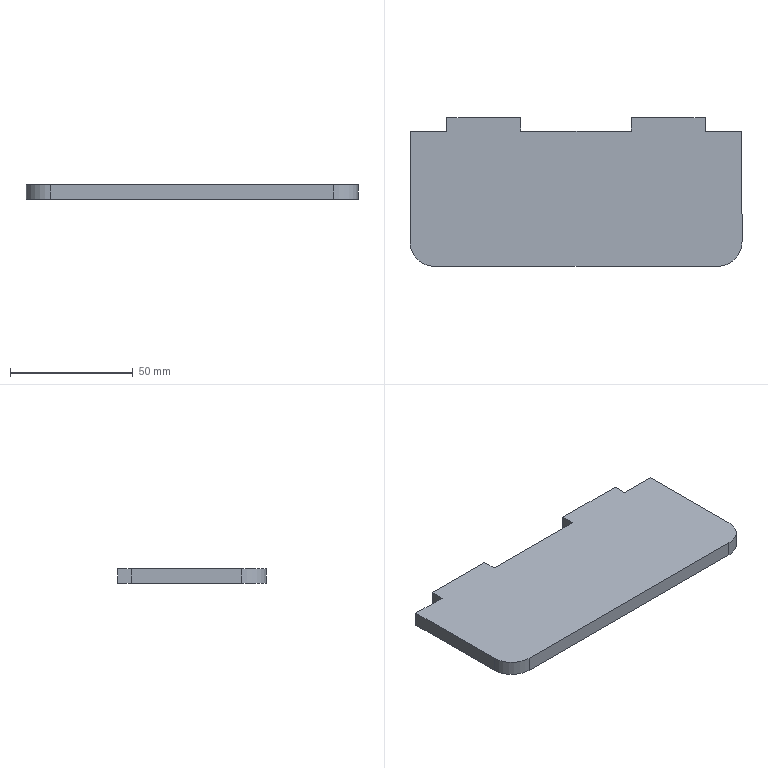Part | SolidWorks | features FlatPattern 1, SMBaseFlange 1, SheetMetal 1 | 1 solid | 16 faces | box 135 x 60.5 x 6 mm | volume 46272 mm3 | plane 14 | cylinder 2 | commonest cylinder face diameters 20 x2
STEP:
#1=CARTESIAN_POINT('',(128.47,-600.5,0.));
#2=VERTEX_POINT('',#1);
#3=CARTESIAN_POINT('',(128.47,-555.5,0.));
#4=VERTEX_POINT('',#3);
#5=CARTESIAN_POINT('',(128.47,-555.5,0.));
#6=DIRECTION('',(0.,1.,0.));
#7=VECTOR('',#6,1000.);
#8=LINE('',#5,#7);
#9=EDGE_CURVE('',#2,#4,#8,.T.);
#10=ORIENTED_EDGE('',*,*,#9,.F.);
#11=CARTESIAN_POINT('',(128.47,-600.5,-6.));
#12=VERTEX_POINT('',#11);
#13=CARTESIAN_POINT('',(128.47,-600.5,-6.));
#14=DIRECTION('',(0.,0.,1.));
#15=VECTOR('',#14,1000.);
#16=LINE('',#13,#15);
#17=EDGE_CURVE('',#12,#2,#16,.T.);
#18=ORIENTED_EDGE('',*,*,#17,.F.);
#19=CARTESIAN_POINT('',(128.47,-555.5,-6.));
#20=VERTEX_POINT('',#19);
#21=CARTESIAN_POINT('',(128.47,-555.5,-6.));
#22=DIRECTION('',(0.,1.,0.));
#23=VECTOR('',#22,1000.);
#24=LINE('',#21,#23);
#25=EDGE_CURVE('',#12,#20,#24,.T.);
#26=ORIENTED_EDGE('',*,*,#25,.T.);
#27=CARTESIAN_POINT('',(128.47,-555.5,-6.));
#28=DIRECTION('',(0.,0.,1.));
#29=VECTOR('',#28,1000.);
#30=LINE('',#27,#29);
#31=EDGE_CURVE('',#20,#4,#30,.T.);
#32=ORIENTED_EDGE('',*,*,#31,.T.);
#33=EDGE_LOOP('',(#10,#18,#26,#32));
#34=FACE_OUTER_BOUND('',#33,.T.);
#35=CARTESIAN_POINT('',(128.47,-555.5,-6.));
#36=DIRECTION('',(1.,0.,0.));
#37=DIRECTION('',(0.,1.,0.));
#38=AXIS2_PLACEMENT_3D('',#35,#36,#37);
#39=PLANE('',#38);
#40=ADVANCED_FACE('',(#34),#39,.T.);
#41=CARTESIAN_POINT('',(118.47,-610.5,0.));
#42=VERTEX_POINT('',#41);
#43=CARTESIAN_POINT('',(118.47,-600.5,0.));
#44=DIRECTION('',(0.,0.,1.));
#45=DIRECTION('',(-1.,0.,0.));
#46=AXIS2_PLACEMENT_3D('',#43,#44,#45);
#47=CIRCLE('',#46,10.);
#48=EDGE_CURVE('',#42,#2,#47,.T.);
#49=ORIENTED_EDGE('',*,*,#48,.F.);
#50=CARTESIAN_POINT('',(118.47,-610.5,-6.));
#51=VERTEX_POINT('',#50);
#52=CARTESIAN_POINT('',(118.47,-610.5,-6.));
#53=DIRECTION('',(0.,0.,1.));
#54=VECTOR('',#53,1000.);
#55=LINE('',#52,#54);
#56=EDGE_CURVE('',#51,#42,#55,.T.);
#57=ORIENTED_EDGE('',*,*,#56,.F.);
#58=CARTESIAN_POINT('',(118.47,-600.5,-6.));
#59=DIRECTION('',(0.,0.,1.));
#60=DIRECTION('',(-1.,0.,0.));
#61=AXIS2_PLACEMENT_3D('',#58,#59,#60);
#62=CIRCLE('',#61,10.);
#63=EDGE_CURVE('',#51,#12,#62,.T.);
#64=ORIENTED_EDGE('',*,*,#63,.T.);
#65=ORIENTED_EDGE('',*,*,#17,.T.);
#66=EDGE_LOOP('',(#49,#57,#64,#65));
#67=FACE_OUTER_BOUND('',#66,.T.);
#68=CARTESIAN_POINT('',(118.47,-600.5,-6.));
#69=DIRECTION('',(0.,0.,1.));
#70=DIRECTION('',(1.,0.,0.));
#71=AXIS2_PLACEMENT_3D('',#68,#69,#70);
#72=CYLINDRICAL_SURFACE('',#71,10.);
#73=ADVANCED_FACE('',(#67),#72,.T.);
#74=CARTESIAN_POINT('',(3.47,-610.5,0.));
#75=VERTEX_POINT('',#74);
#76=CARTESIAN_POINT('',(118.47,-610.5,0.));
#77=DIRECTION('',(1.,0.,0.));
#78=VECTOR('',#77,1000.);
#79=LINE('',#76,#78);
#80=EDGE_CURVE('',#75,#42,#79,.T.);
#81=ORIENTED_EDGE('',*,*,#80,.F.);
#82=CARTESIAN_POINT('',(3.47,-610.5,-6.));
#83=VERTEX_POINT('',#82);
#84=CARTESIAN_POINT('',(3.47,-610.5,-6.));
#85=DIRECTION('',(0.,0.,1.));
#86=VECTOR('',#85,1000.);
#87=LINE('',#84,#86);
#88=EDGE_CURVE('',#83,#75,#87,.T.);
#89=ORIENTED_EDGE('',*,*,#88,.F.);
#90=CARTESIAN_POINT('',(118.47,-610.5,-6.));
#91=DIRECTION('',(1.,0.,0.));
#92=VECTOR('',#91,1000.);
#93=LINE('',#90,#92);
#94=EDGE_CURVE('',#83,#51,#93,.T.);
#95=ORIENTED_EDGE('',*,*,#94,.T.);
#96=ORIENTED_EDGE('',*,*,#56,.T.);
#97=EDGE_LOOP('',(#81,#89,#95,#96));
#98=FACE_OUTER_BOUND('',#97,.T.);
#99=CARTESIAN_POINT('',(118.47,-610.5,-6.));
#100=DIRECTION('',(0.,-1.,0.));
#101=DIRECTION('',(1.,0.,0.));
#102=AXIS2_PLACEMENT_3D('',#99,#100,#101);
#103=PLANE('',#102);
#104=ADVANCED_FACE('',(#98),#103,.T.);
#105=CARTESIAN_POINT('',(-6.53,-600.5,0.));
#106=VERTEX_POINT('',#105);
#107=CARTESIAN_POINT('',(3.47,-600.5,0.));
#108=DIRECTION('',(0.,0.,1.));
#109=DIRECTION('',(-1.,0.,0.));
#110=AXIS2_PLACEMENT_3D('',#107,#108,#109);
#111=CIRCLE('',#110,10.);
#112=EDGE_CURVE('',#106,#75,#111,.T.);
#113=ORIENTED_EDGE('',*,*,#112,.F.);
#114=CARTESIAN_POINT('',(-6.53,-600.5,-6.));
#115=VERTEX_POINT('',#114);
#116=CARTESIAN_POINT('',(-6.53,-600.5,-6.));
#117=DIRECTION('',(0.,0.,1.));
#118=VECTOR('',#117,1000.);
#119=LINE('',#116,#118);
#120=EDGE_CURVE('',#115,#106,#119,.T.);
#121=ORIENTED_EDGE('',*,*,#120,.F.);
#122=CARTESIAN_POINT('',(3.47,-600.5,-6.));
#123=DIRECTION('',(0.,0.,1.));
#124=DIRECTION('',(-1.,0.,0.));
#125=AXIS2_PLACEMENT_3D('',#122,#123,#124);
#126=CIRCLE('',#125,10.);
#127=EDGE_CURVE('',#115,#83,#126,.T.);
#128=ORIENTED_EDGE('',*,*,#127,.T.);
#129=ORIENTED_EDGE('',*,*,#88,.T.);
#130=EDGE_LOOP('',(#113,#121,#128,#129));
#131=FACE_OUTER_BOUND('',#130,.T.);
#132=CARTESIAN_POINT('',(3.47,-600.5,-6.));
#133=DIRECTION('',(0.,0.,1.));
#134=DIRECTION('',(1.,0.,0.));
#135=AXIS2_PLACEMENT_3D('',#132,#133,#134);
#136=CYLINDRICAL_SURFACE('',#135,10.);
#137=ADVANCED_FACE('',(#131),#136,.T.);
#138=CARTESIAN_POINT('',(-6.53,-555.5,0.));
#139=VERTEX_POINT('',#138);
#140=CARTESIAN_POINT('',(-6.53,-555.5,0.));
#141=DIRECTION('',(0.,-1.,0.));
#142=VECTOR('',#141,1000.);
#143=LINE('',#140,#142);
#144=EDGE_CURVE('',#139,#106,#143,.T.);
#145=ORIENTED_EDGE('',*,*,#144,.F.);
#146=CARTESIAN_POINT('',(-6.53,-555.5,-6.));
#147=VERTEX_POINT('',#146);
#148=CARTESIAN_POINT('',(-6.53,-555.5,-6.));
#149=DIRECTION('',(0.,0.,1.));
#150=VECTOR('',#149,1000.);
#151=LINE('',#148,#150);
#152=EDGE_CURVE('',#147,#139,#151,.T.);
#153=ORIENTED_EDGE('',*,*,#152,.F.);
#154=CARTESIAN_POINT('',(-6.53,-555.5,-6.));
#155=DIRECTION('',(0.,-1.,0.));
#156=VECTOR('',#155,1000.);
#157=LINE('',#154,#156);
#158=EDGE_CURVE('',#147,#115,#157,.T.);
#159=ORIENTED_EDGE('',*,*,#158,.T.);
#160=ORIENTED_EDGE('',*,*,#120,.T.);
#161=EDGE_LOOP('',(#145,#153,#159,#160));
#162=FACE_OUTER_BOUND('',#161,.T.);
#163=CARTESIAN_POINT('',(-6.53,-555.5,-6.));
#164=DIRECTION('',(-1.,0.,0.));
#165=DIRECTION('',(0.,-1.,0.));
#166=AXIS2_PLACEMENT_3D('',#163,#164,#165);
#167=PLANE('',#166);
#168=ADVANCED_FACE('',(#162),#167,.T.);
#169=CARTESIAN_POINT('',(8.47,-555.5,0.));
#170=VERTEX_POINT('',#169);
#171=CARTESIAN_POINT('',(8.47,-555.5,0.));
#172=DIRECTION('',(-1.,0.,0.));
#173=VECTOR('',#172,1000.);
#174=LINE('',#171,#173);
#175=EDGE_CURVE('',#170,#139,#174,.T.);
#176=ORIENTED_EDGE('',*,*,#175,.F.);
#177=CARTESIAN_POINT('',(8.47,-555.5,-6.));
#178=VERTEX_POINT('',#177);
#179=CARTESIAN_POINT('',(8.47,-555.5,-6.));
#180=DIRECTION('',(0.,0.,1.));
#181=VECTOR('',#180,1000.);
#182=LINE('',#179,#181);
#183=EDGE_CURVE('',#178,#170,#182,.T.);
#184=ORIENTED_EDGE('',*,*,#183,.F.);
#185=CARTESIAN_POINT('',(8.47,-555.5,-6.));
#186=DIRECTION('',(-1.,0.,0.));
#187=VECTOR('',#186,1000.);
#188=LINE('',#185,#187);
#189=EDGE_CURVE('',#178,#147,#188,.T.);
#190=ORIENTED_EDGE('',*,*,#189,.T.);
#191=ORIENTED_EDGE('',*,*,#152,.T.);
#192=EDGE_LOOP('',(#176,#184,#190,#191));
#193=FACE_OUTER_BOUND('',#192,.T.);
#194=CARTESIAN_POINT('',(8.47,-555.5,-6.));
#195=DIRECTION('',(0.,1.,0.));
#196=DIRECTION('',(0.,0.,1.));
#197=AXIS2_PLACEMENT_3D('',#194,#195,#196);
#198=PLANE('',#197);
#199=ADVANCED_FACE('',(#193),#198,.T.);
#200=CARTESIAN_POINT('',(8.47,-550.,0.));
#201=VERTEX_POINT('',#200);
#202=CARTESIAN_POINT('',(8.47,-550.,0.));
#203=DIRECTION('',(0.,-1.,0.));
#204=VECTOR('',#203,1000.);
#205=LINE('',#202,#204);
#206=EDGE_CURVE('',#201,#170,#205,.T.);
#207=ORIENTED_EDGE('',*,*,#206,.F.);
#208=CARTESIAN_POINT('',(8.47,-550.,-6.));
#209=VERTEX_POINT('',#208);
#210=CARTESIAN_POINT('',(8.47,-550.,-6.));
#211=DIRECTION('',(0.,0.,1.));
#212=VECTOR('',#211,1000.);
#213=LINE('',#210,#212);
#214=EDGE_CURVE('',#209,#201,#213,.T.);
#215=ORIENTED_EDGE('',*,*,#214,.F.);
#216=CARTESIAN_POINT('',(8.47,-550.,-6.));
#217=DIRECTION('',(0.,-1.,0.));
#218=VECTOR('',#217,1000.);
#219=LINE('',#216,#218);
#220=EDGE_CURVE('',#209,#178,#219,.T.);
#221=ORIENTED_EDGE('',*,*,#220,.T.);
#222=ORIENTED_EDGE('',*,*,#183,.T.);
#223=EDGE_LOOP('',(#207,#215,#221,#222));
#224=FACE_OUTER_BOUND('',#223,.T.);
#225=CARTESIAN_POINT('',(8.47,-550.,-6.));
#226=DIRECTION('',(-1.,0.,0.));
#227=DIRECTION('',(0.,0.,1.));
#228=AXIS2_PLACEMENT_3D('',#225,#226,#227);
#229=PLANE('',#228);
#230=ADVANCED_FACE('',(#224),#229,.T.);
#231=CARTESIAN_POINT('',(38.47,-550.,0.));
#232=VERTEX_POINT('',#231);
#233=CARTESIAN_POINT('',(38.47,-550.,0.));
#234=DIRECTION('',(-1.,0.,0.));
#235=VECTOR('',#234,1000.);
#236=LINE('',#233,#235);
#237=EDGE_CURVE('',#232,#201,#236,.T.);
#238=ORIENTED_EDGE('',*,*,#237,.F.);
#239=CARTESIAN_POINT('',(38.47,-550.,-6.));
#240=VERTEX_POINT('',#239);
#241=CARTESIAN_POINT('',(38.47,-550.,-6.));
#242=DIRECTION('',(0.,0.,1.));
#243=VECTOR('',#242,1000.);
#244=LINE('',#241,#243);
#245=EDGE_CURVE('',#240,#232,#244,.T.);
#246=ORIENTED_EDGE('',*,*,#245,.F.);
#247=CARTESIAN_POINT('',(38.47,-550.,-6.));
#248=DIRECTION('',(-1.,0.,0.));
#249=VECTOR('',#248,1000.);
#250=LINE('',#247,#249);
#251=EDGE_CURVE('',#240,#209,#250,.T.);
#252=ORIENTED_EDGE('',*,*,#251,.T.);
#253=ORIENTED_EDGE('',*,*,#214,.T.);
#254=EDGE_LOOP('',(#238,#246,#252,#253));
#255=FACE_OUTER_BOUND('',#254,.T.);
#256=CARTESIAN_POINT('',(38.47,-550.,-6.));
#257=DIRECTION('',(0.,1.,0.));
#258=DIRECTION('',(0.,0.,1.));
#259=AXIS2_PLACEMENT_3D('',#256,#257,#258);
#260=PLANE('',#259);
#261=ADVANCED_FACE('',(#255),#260,.T.);
#262=CARTESIAN_POINT('',(38.47,-555.5,0.));
#263=VERTEX_POINT('',#262);
#264=CARTESIAN_POINT('',(38.47,-555.5,0.));
#265=DIRECTION('',(0.,1.,0.));
#266=VECTOR('',#265,1000.);
#267=LINE('',#264,#266);
#268=EDGE_CURVE('',#263,#232,#267,.T.);
#269=ORIENTED_EDGE('',*,*,#268,.F.);
#270=CARTESIAN_POINT('',(38.47,-555.5,-6.));
#271=VERTEX_POINT('',#270);
#272=CARTESIAN_POINT('',(38.47,-555.5,-6.));
#273=DIRECTION('',(0.,0.,1.));
#274=VECTOR('',#273,1000.);
#275=LINE('',#272,#274);
#276=EDGE_CURVE('',#271,#263,#275,.T.);
#277=ORIENTED_EDGE('',*,*,#276,.F.);
#278=CARTESIAN_POINT('',(38.47,-555.5,-6.));
#279=DIRECTION('',(0.,1.,0.));
#280=VECTOR('',#279,1000.);
#281=LINE('',#278,#280);
#282=EDGE_CURVE('',#271,#240,#281,.T.);
#283=ORIENTED_EDGE('',*,*,#282,.T.);
#284=ORIENTED_EDGE('',*,*,#245,.T.);
#285=EDGE_LOOP('',(#269,#277,#283,#284));
#286=FACE_OUTER_BOUND('',#285,.T.);
#287=CARTESIAN_POINT('',(38.47,-555.5,-6.));
#288=DIRECTION('',(1.,0.,0.));
#289=DIRECTION('',(0.,0.,-1.));
#290=AXIS2_PLACEMENT_3D('',#287,#288,#289);
#291=PLANE('',#290);
#292=ADVANCED_FACE('',(#286),#291,.T.);
#293=CARTESIAN_POINT('',(83.47,-555.5,0.));
#294=VERTEX_POINT('',#293);
#295=CARTESIAN_POINT('',(83.47,-555.5,0.));
#296=DIRECTION('',(-1.,0.,0.));
#297=VECTOR('',#296,1000.);
#298=LINE('',#295,#297);
#299=EDGE_CURVE('',#294,#263,#298,.T.);
#300=ORIENTED_EDGE('',*,*,#299,.F.);
#301=CARTESIAN_POINT('',(83.47,-555.5,-6.));
#302=VERTEX_POINT('',#301);
#303=CARTESIAN_POINT('',(83.47,-555.5,-6.));
#304=DIRECTION('',(0.,0.,1.));
#305=VECTOR('',#304,1000.);
#306=LINE('',#303,#305);
#307=EDGE_CURVE('',#302,#294,#306,.T.);
#308=ORIENTED_EDGE('',*,*,#307,.F.);
#309=CARTESIAN_POINT('',(83.47,-555.5,-6.));
#310=DIRECTION('',(-1.,0.,0.));
#311=VECTOR('',#310,1000.);
#312=LINE('',#309,#311);
#313=EDGE_CURVE('',#302,#271,#312,.T.);
#314=ORIENTED_EDGE('',*,*,#313,.T.);
#315=ORIENTED_EDGE('',*,*,#276,.T.);
#316=EDGE_LOOP('',(#300,#308,#314,#315));
#317=FACE_OUTER_BOUND('',#316,.T.);
#318=CARTESIAN_POINT('',(83.47,-555.5,-6.));
#319=DIRECTION('',(0.,1.,0.));
#320=DIRECTION('',(0.,0.,1.));
#321=AXIS2_PLACEMENT_3D('',#318,#319,#320);
#322=PLANE('',#321);
#323=ADVANCED_FACE('',(#317),#322,.T.);
#324=CARTESIAN_POINT('',(83.47,-550.,0.));
#325=VERTEX_POINT('',#324);
#326=CARTESIAN_POINT('',(83.47,-550.,0.));
#327=DIRECTION('',(0.,-1.,0.));
#328=VECTOR('',#327,1000.);
#329=LINE('',#326,#328);
#330=EDGE_CURVE('',#325,#294,#329,.T.);
#331=ORIENTED_EDGE('',*,*,#330,.F.);
#332=CARTESIAN_POINT('',(83.47,-550.,-6.));
#333=VERTEX_POINT('',#332);
#334=CARTESIAN_POINT('',(83.47,-550.,-6.));
#335=DIRECTION('',(0.,0.,1.));
#336=VECTOR('',#335,1000.);
#337=LINE('',#334,#336);
#338=EDGE_CURVE('',#333,#325,#337,.T.);
#339=ORIENTED_EDGE('',*,*,#338,.F.);
#340=CARTESIAN_POINT('',(83.47,-550.,-6.));
#341=DIRECTION('',(0.,-1.,0.));
#342=VECTOR('',#341,1000.);
#343=LINE('',#340,#342);
#344=EDGE_CURVE('',#333,#302,#343,.T.);
#345=ORIENTED_EDGE('',*,*,#344,.T.);
#346=ORIENTED_EDGE('',*,*,#307,.T.);
#347=EDGE_LOOP('',(#331,#339,#345,#346));
#348=FACE_OUTER_BOUND('',#347,.T.);
#349=CARTESIAN_POINT('',(83.47,-550.,-6.));
#350=DIRECTION('',(-1.,0.,0.));
#351=DIRECTION('',(0.,0.,1.));
#352=AXIS2_PLACEMENT_3D('',#349,#350,#351);
#353=PLANE('',#352);
#354=ADVANCED_FACE('',(#348),#353,.T.);
#355=CARTESIAN_POINT('',(113.47,-550.,0.));
#356=VERTEX_POINT('',#355);
#357=CARTESIAN_POINT('',(113.47,-550.,0.));
#358=DIRECTION('',(-1.,0.,0.));
#359=VECTOR('',#358,1000.);
#360=LINE('',#357,#359);
#361=EDGE_CURVE('',#356,#325,#360,.T.);
#362=ORIENTED_EDGE('',*,*,#361,.F.);
#363=CARTESIAN_POINT('',(113.47,-550.,-6.));
#364=VERTEX_POINT('',#363);
#365=CARTESIAN_POINT('',(113.47,-550.,-6.));
#366=DIRECTION('',(0.,0.,1.));
#367=VECTOR('',#366,1000.);
#368=LINE('',#365,#367);
#369=EDGE_CURVE('',#364,#356,#368,.T.);
#370=ORIENTED_EDGE('',*,*,#369,.F.);
#371=CARTESIAN_POINT('',(113.47,-550.,-6.));
#372=DIRECTION('',(-1.,0.,0.));
#373=VECTOR('',#372,1000.);
#374=LINE('',#371,#373);
#375=EDGE_CURVE('',#364,#333,#374,.T.);
#376=ORIENTED_EDGE('',*,*,#375,.T.);
#377=ORIENTED_EDGE('',*,*,#338,.T.);
#378=EDGE_LOOP('',(#362,#370,#376,#377));
#379=FACE_OUTER_BOUND('',#378,.T.);
#380=CARTESIAN_POINT('',(113.47,-550.,-6.));
#381=DIRECTION('',(0.,1.,0.));
#382=DIRECTION('',(0.,0.,1.));
#383=AXIS2_PLACEMENT_3D('',#380,#381,#382);
#384=PLANE('',#383);
#385=ADVANCED_FACE('',(#379),#384,.T.);
#386=CARTESIAN_POINT('',(113.47,-555.5,0.));
#387=VERTEX_POINT('',#386);
#388=CARTESIAN_POINT('',(113.47,-555.5,0.));
#389=DIRECTION('',(0.,1.,0.));
#390=VECTOR('',#389,1000.);
#391=LINE('',#388,#390);
#392=EDGE_CURVE('',#387,#356,#391,.T.);
#393=ORIENTED_EDGE('',*,*,#392,.F.);
#394=CARTESIAN_POINT('',(113.47,-555.5,-6.));
#395=VERTEX_POINT('',#394);
#396=CARTESIAN_POINT('',(113.47,-555.5,-6.));
#397=DIRECTION('',(0.,0.,1.));
#398=VECTOR('',#397,1000.);
#399=LINE('',#396,#398);
#400=EDGE_CURVE('',#395,#387,#399,.T.);
#401=ORIENTED_EDGE('',*,*,#400,.F.);
#402=CARTESIAN_POINT('',(113.47,-555.5,-6.));
#403=DIRECTION('',(0.,1.,0.));
#404=VECTOR('',#403,1000.);
#405=LINE('',#402,#404);
#406=EDGE_CURVE('',#395,#364,#405,.T.);
#407=ORIENTED_EDGE('',*,*,#406,.T.);
#408=ORIENTED_EDGE('',*,*,#369,.T.);
#409=EDGE_LOOP('',(#393,#401,#407,#408));
#410=FACE_OUTER_BOUND('',#409,.T.);
#411=CARTESIAN_POINT('',(113.47,-555.5,-6.));
#412=DIRECTION('',(1.,0.,0.));
#413=DIRECTION('',(0.,0.,-1.));
#414=AXIS2_PLACEMENT_3D('',#411,#412,#413);
#415=PLANE('',#414);
#416=ADVANCED_FACE('',(#410),#415,.T.);
#417=CARTESIAN_POINT('',(128.47,-555.5,0.));
#418=DIRECTION('',(-1.,0.,0.));
#419=VECTOR('',#418,1000.);
#420=LINE('',#417,#419);
#421=EDGE_CURVE('',#4,#387,#420,.T.);
#422=ORIENTED_EDGE('',*,*,#421,.F.);
#423=ORIENTED_EDGE('',*,*,#31,.F.);
#424=CARTESIAN_POINT('',(128.47,-555.5,-6.));
#425=DIRECTION('',(-1.,0.,0.));
#426=VECTOR('',#425,1000.);
#427=LINE('',#424,#426);
#428=EDGE_CURVE('',#20,#395,#427,.T.);
#429=ORIENTED_EDGE('',*,*,#428,.T.);
#430=ORIENTED_EDGE('',*,*,#400,.T.);
#431=EDGE_LOOP('',(#422,#423,#429,#430));
#432=FACE_OUTER_BOUND('',#431,.T.);
#433=CARTESIAN_POINT('',(128.47,-555.5,-6.));
#434=DIRECTION('',(0.,1.,0.));
#435=DIRECTION('',(0.,0.,1.));
#436=AXIS2_PLACEMENT_3D('',#433,#434,#435);
#437=PLANE('',#436);
#438=ADVANCED_FACE('',(#432),#437,.T.);
#439=ORIENTED_EDGE('',*,*,#25,.F.);
#440=ORIENTED_EDGE('',*,*,#63,.F.);
#441=ORIENTED_EDGE('',*,*,#94,.F.);
#442=ORIENTED_EDGE('',*,*,#127,.F.);
#443=ORIENTED_EDGE('',*,*,#158,.F.);
#444=ORIENTED_EDGE('',*,*,#189,.F.);
#445=ORIENTED_EDGE('',*,*,#220,.F.);
#446=ORIENTED_EDGE('',*,*,#251,.F.);
#447=ORIENTED_EDGE('',*,*,#282,.F.);
#448=ORIENTED_EDGE('',*,*,#313,.F.);
#449=ORIENTED_EDGE('',*,*,#344,.F.);
#450=ORIENTED_EDGE('',*,*,#375,.F.);
#451=ORIENTED_EDGE('',*,*,#406,.F.);
#452=ORIENTED_EDGE('',*,*,#428,.F.);
#453=EDGE_LOOP('',(#439,#440,#441,#442,#443,#444,#445,#446,#447,#448,#449,#450,#451,#452));
#454=FACE_OUTER_BOUND('',#453,.T.);
#455=CARTESIAN_POINT('',(118.47,-600.5,-6.));
#456=DIRECTION('',(0.,0.,-1.));
#457=DIRECTION('',(-1.,0.,0.));
#458=AXIS2_PLACEMENT_3D('',#455,#456,#457);
#459=PLANE('',#458);
#460=ADVANCED_FACE('',(#454),#459,.T.);
#461=ORIENTED_EDGE('',*,*,#9,.T.);
#462=ORIENTED_EDGE('',*,*,#421,.T.);
#463=ORIENTED_EDGE('',*,*,#392,.T.);
#464=ORIENTED_EDGE('',*,*,#361,.T.);
#465=ORIENTED_EDGE('',*,*,#330,.T.);
#466=ORIENTED_EDGE('',*,*,#299,.T.);
#467=ORIENTED_EDGE('',*,*,#268,.T.);
#468=ORIENTED_EDGE('',*,*,#237,.T.);
#469=ORIENTED_EDGE('',*,*,#206,.T.);
#470=ORIENTED_EDGE('',*,*,#175,.T.);
#471=ORIENTED_EDGE('',*,*,#144,.T.);
#472=ORIENTED_EDGE('',*,*,#112,.T.);
#473=ORIENTED_EDGE('',*,*,#80,.T.);
#474=ORIENTED_EDGE('',*,*,#48,.T.);
#475=EDGE_LOOP('',(#461,#462,#463,#464,#465,#466,#467,#468,#469,#470,#471,#472,#473,#474));
#476=FACE_OUTER_BOUND('',#475,.T.);
#477=CARTESIAN_POINT('',(118.47,-600.5,0.));
#478=DIRECTION('',(0.,0.,-1.));
#479=DIRECTION('',(-1.,0.,0.));
#480=AXIS2_PLACEMENT_3D('',#477,#478,#479);
#481=PLANE('',#480);
#482=ADVANCED_FACE('',(#476),#481,.F.);
#483=CLOSED_SHELL('',(#40,#73,#104,#137,#168,#199,#230,#261,#292,#323,#354,#385,#416,#438,#460,#482));
#484=MANIFOLD_SOLID_BREP('',#483);
#485=CARTESIAN_POINT('',(0.,0.,0.));
#486=DIRECTION('',(0.,0.,1.));
#487=DIRECTION('',(1.,0.,0.));
#488=AXIS2_PLACEMENT_3D('',#485,#486,#487);
#489=(LENGTH_UNIT()NAMED_UNIT(*)SI_UNIT(.MILLI.,.METRE.));
#490=UNCERTAINTY_MEASURE_WITH_UNIT(LENGTH_MEASURE(0.00001),#489,'','');
#491=(NAMED_UNIT(*)PLANE_ANGLE_UNIT()SI_UNIT($,.RADIAN.));
#492=(NAMED_UNIT(*)SI_UNIT($,.STERADIAN.)SOLID_ANGLE_UNIT());
#493=(GEOMETRIC_REPRESENTATION_CONTEXT(3)GLOBAL_UNCERTAINTY_ASSIGNED_CONTEXT((#490))GLOBAL_UNIT_ASSIGNED_CONTEXT((#489,#491,#492))REPRESENTATION_CONTEXT('',''));
#494=ADVANCED_BREP_SHAPE_REPRESENTATION('',(#484,#488),#493);